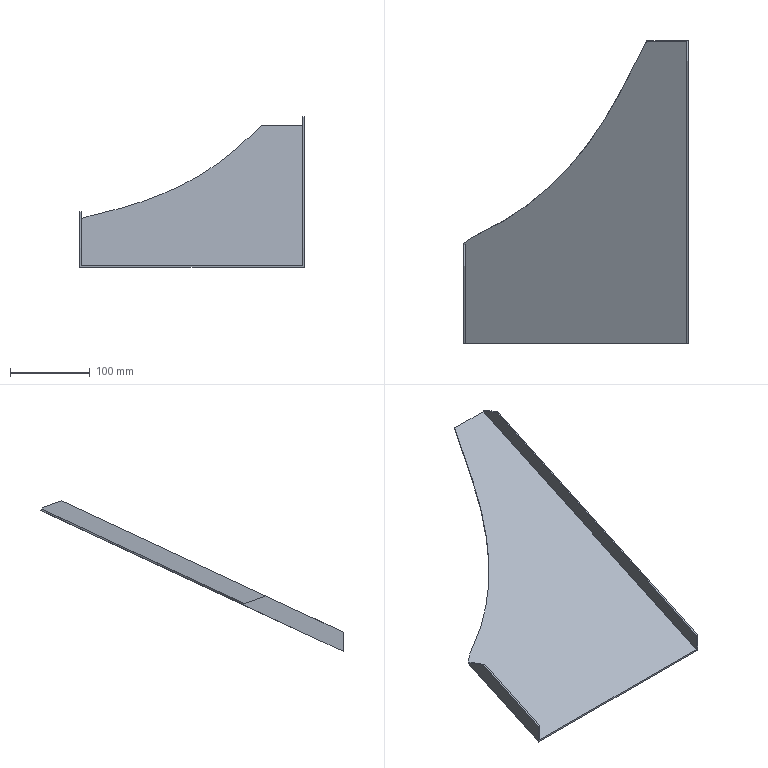Part | NX | features solid 2 | 1 solid | 13 faces | box 282.306 x 379.378 x 189.239 mm | volume 176482 mm3 | plane 12 | spline 1
STEP:
#1=CARTESIAN_POINT('',(299.694,-556.33,-245.421));
#2=VERTEX_POINT('',#1);
#3=CARTESIAN_POINT('',(297.694,-556.33,-245.421));
#4=VERTEX_POINT('',#3);
#5=CARTESIAN_POINT('',(337.694,-556.33,-245.421));
#6=DIRECTION('',(1.,0.,0.));
#7=VECTOR('',#6,1000.);
#8=LINE('',#5,#7);
#9=EDGE_CURVE('',#2,#4,#8,.F.);
#10=ORIENTED_EDGE('',*,*,#9,.F.);
#11=CARTESIAN_POINT('',(299.694,-680.,-303.09));
#12=VERTEX_POINT('',#11);
#13=CARTESIAN_POINT('',(299.694,-522.729,-229.753));
#14=DIRECTION('',(0.,-0.9063,-0.4226));
#15=VECTOR('',#14,1000.);
#16=LINE('',#13,#15);
#17=EDGE_CURVE('',#2,#12,#16,.T.);
#18=ORIENTED_EDGE('',*,*,#17,.T.);
#19=CARTESIAN_POINT('',(578.,-680.,-303.09));
#20=VERTEX_POINT('',#19);
#21=CARTESIAN_POINT('',(188.564,-680.,-303.09));
#22=DIRECTION('',(1.,0.,0.));
#23=VECTOR('',#22,1000.);
#24=LINE('',#21,#23);
#25=EDGE_CURVE('',#20,#12,#24,.F.);
#26=ORIENTED_EDGE('',*,*,#25,.F.);
#27=CARTESIAN_POINT('',(578.,-301.467,-126.577));
#28=VERTEX_POINT('',#27);
#29=CARTESIAN_POINT('',(578.,-522.729,-229.753));
#30=DIRECTION('',(0.,-0.9063,-0.4226));
#31=VECTOR('',#30,1000.);
#32=LINE('',#29,#31);
#33=EDGE_CURVE('',#28,#20,#32,.T.);
#34=ORIENTED_EDGE('',*,*,#33,.F.);
#35=CARTESIAN_POINT('',(527.431,-301.467,-126.577));
#36=VERTEX_POINT('',#35);
#37=CARTESIAN_POINT('',(570.,-301.467,-126.577));
#38=DIRECTION('',(-1.,0.,0.));
#39=VECTOR('',#38,1000.);
#40=LINE('',#37,#39);
#41=EDGE_CURVE('',#28,#36,#40,.T.);
#42=ORIENTED_EDGE('',*,*,#41,.T.);
#43=CARTESIAN_POINT('',(297.694,-555.03,-244.815));
#44=VERTEX_POINT('',#43);
#45=CARTESIAN_POINT('',(527.431,-301.467,-126.577));
#46=CARTESIAN_POINT('',(520.866,-314.161,-132.496));
#47=CARTESIAN_POINT('',(510.995,-333.189,-141.369));
#48=CARTESIAN_POINT('',(497.924,-358.611,-153.224));
#49=CARTESIAN_POINT('',(484.556,-383.863,-164.999));
#50=CARTESIAN_POINT('',(465.949,-414.249,-179.168));
#51=CARTESIAN_POINT('',(440.229,-448.639,-195.204));
#52=CARTESIAN_POINT('',(415.403,-475.145,-207.565));
#53=CARTESIAN_POINT('',(393.073,-494.953,-216.801));
#54=CARTESIAN_POINT('',(375.401,-508.723,-223.222));
#55=CARTESIAN_POINT('',(356.832,-521.362,-229.116));
#56=CARTESIAN_POINT('',(340.563,-530.912,-233.569));
#57=CARTESIAN_POINT('',(327.082,-537.971,-236.861));
#58=CARTESIAN_POINT('',(316.711,-542.944,-239.18));
#59=CARTESIAN_POINT('',(308.204,-547.256,-241.19));
#60=CARTESIAN_POINT('',(302.245,-551.756,-243.289));
#61=CARTESIAN_POINT('',(299.206,-553.933,-244.304));
#62=CARTESIAN_POINT('',(297.694,-555.03,-244.815));
#63=B_SPLINE_CURVE_WITH_KNOTS('',3,(#45,#46,#47,#48,#49,#50,#51,#52,#53,#54,#55,#56,#57,#58,#59,#60,#61,#62),.UNSPECIFIED.,.F.,.F.,(4,1,1,1,1,1,1,1,1,1,1,1,1,1,1,4),(0.9959,1.042,1.065,1.089,1.135,1.182,1.228,1.251,1.274,1.298,1.321,1.332,1.344,1.356,1.361,1.367),.UNSPECIFIED.);
#64=EDGE_CURVE('',#36,#44,#63,.T.);
#65=ORIENTED_EDGE('',*,*,#64,.T.);
#66=CARTESIAN_POINT('',(297.694,-522.729,-229.753));
#67=DIRECTION('',(0.,0.9063,0.4226));
#68=VECTOR('',#67,1000.);
#69=LINE('',#66,#68);
#70=EDGE_CURVE('',#4,#44,#69,.T.);
#71=ORIENTED_EDGE('',*,*,#70,.F.);
#72=EDGE_LOOP('',(#10,#18,#26,#34,#42,#65,#71));
#73=FACE_BOUND('',#72,.T.);
#74=CARTESIAN_POINT('',(337.694,-522.729,-229.753));
#75=DIRECTION('',(0.,-0.4226,0.9063));
#76=DIRECTION('',(1.,0.,0.));
#77=AXIS2_PLACEMENT_3D('',#74,#75,#76);
#78=PLANE('',#77);
#79=ADVANCED_FACE('',(#73),#78,.T.);
#80=CARTESIAN_POINT('',(578.,-302.312,-124.764));
#81=VERTEX_POINT('',#80);
#82=CARTESIAN_POINT('',(578.,-301.467,-126.577));
#83=DIRECTION('',(0.,-0.4226,0.9063));
#84=VECTOR('',#83,1000.);
#85=LINE('',#82,#84);
#86=EDGE_CURVE('',#28,#81,#85,.T.);
#87=ORIENTED_EDGE('',*,*,#86,.T.);
#88=CARTESIAN_POINT('',(580.,-302.312,-124.764));
#89=VERTEX_POINT('',#88);
#90=CARTESIAN_POINT('',(570.,-302.312,-124.764));
#91=DIRECTION('',(1.,0.,0.));
#92=VECTOR('',#91,1000.);
#93=LINE('',#90,#92);
#94=EDGE_CURVE('',#81,#89,#93,.T.);
#95=ORIENTED_EDGE('',*,*,#94,.T.);
#96=CARTESIAN_POINT('',(580.,-300.622,-128.389));
#97=VERTEX_POINT('',#96);
#98=CARTESIAN_POINT('',(580.,-301.467,-126.577));
#99=DIRECTION('',(0.,0.4226,-0.9063));
#100=VECTOR('',#99,1000.);
#101=LINE('',#98,#100);
#102=EDGE_CURVE('',#89,#97,#101,.T.);
#103=ORIENTED_EDGE('',*,*,#102,.T.);
#104=CARTESIAN_POINT('',(527.869,-300.622,-128.389));
#105=VERTEX_POINT('',#104);
#106=CARTESIAN_POINT('',(570.,-300.622,-128.389));
#107=DIRECTION('',(-1.,0.,0.));
#108=VECTOR('',#107,1000.);
#109=LINE('',#106,#108);
#110=EDGE_CURVE('',#97,#105,#109,.T.);
#111=ORIENTED_EDGE('',*,*,#110,.T.);
#112=CARTESIAN_POINT('',(527.431,-301.467,-126.577));
#113=CARTESIAN_POINT('',(527.577,-301.185,-127.181));
#114=CARTESIAN_POINT('',(527.723,-300.903,-127.785));
#115=CARTESIAN_POINT('',(527.869,-300.622,-128.389));
#116=B_SPLINE_CURVE_WITH_KNOTS('',3,(#112,#113,#114,#115),.UNSPECIFIED.,.F.,.F.,(4,4),(0.07876,0.08081),.UNSPECIFIED.);
#117=EDGE_CURVE('',#36,#105,#116,.T.);
#118=ORIENTED_EDGE('',*,*,#117,.F.);
#119=ORIENTED_EDGE('',*,*,#41,.F.);
#120=EDGE_LOOP('',(#87,#95,#103,#111,#118,#119));
#121=FACE_BOUND('',#120,.T.);
#122=CARTESIAN_POINT('',(570.,-301.467,-126.577));
#123=DIRECTION('',(0.,-0.9063,-0.4226));
#124=DIRECTION('',(0.,0.4226,-0.9063));
#125=AXIS2_PLACEMENT_3D('',#122,#123,#124);
#126=PLANE('',#125);
#127=ADVANCED_FACE('',(#121),#126,.F.);
#128=CARTESIAN_POINT('',(297.694,-555.03,-247.022));
#129=VERTEX_POINT('',#128);
#130=CARTESIAN_POINT('',(527.869,-300.622,-128.389));
#131=CARTESIAN_POINT('',(521.294,-313.334,-134.317));
#132=CARTESIAN_POINT('',(511.409,-332.39,-143.203));
#133=CARTESIAN_POINT('',(498.317,-357.846,-155.074));
#134=CARTESIAN_POINT('',(484.961,-383.152,-166.874));
#135=CARTESIAN_POINT('',(466.378,-413.617,-181.08));
#136=CARTESIAN_POINT('',(440.678,-448.104,-197.161));
#137=CARTESIAN_POINT('',(415.858,-474.699,-209.563));
#138=CARTESIAN_POINT('',(393.532,-494.571,-218.83));
#139=CARTESIAN_POINT('',(375.839,-508.405,-225.281));
#140=CARTESIAN_POINT('',(357.211,-521.124,-231.212));
#141=CARTESIAN_POINT('',(340.857,-530.75,-235.7));
#142=CARTESIAN_POINT('',(327.286,-537.87,-239.02));
#143=CARTESIAN_POINT('',(316.84,-542.884,-241.358));
#144=CARTESIAN_POINT('',(308.261,-547.216,-243.378));
#145=CARTESIAN_POINT('',(302.27,-551.738,-245.487));
#146=CARTESIAN_POINT('',(299.214,-553.927,-246.508));
#147=CARTESIAN_POINT('',(297.694,-555.03,-247.022));
#148=B_SPLINE_CURVE_WITH_KNOTS('',3,(#130,#131,#132,#133,#134,#135,#136,#137,#138,#139,#140,#141,#142,#143,#144,#145,#146,#147),.UNSPECIFIED.,.F.,.F.,(4,1,1,1,1,1,1,1,1,1,1,1,1,1,1,4),(-0.06545,-0.01955,0.003406,0.02636,0.07226,0.1182,0.1641,0.187,0.21,0.2329,0.2559,0.2674,0.2788,0.2903,0.2961,0.3018),.UNSPECIFIED.);
#149=EDGE_CURVE('',#105,#129,#148,.T.);
#150=ORIENTED_EDGE('',*,*,#149,.T.);
#151=CARTESIAN_POINT('',(297.694,-555.03,-235.335));
#152=DIRECTION('',(0.,0.,1.));
#153=VECTOR('',#152,1000.);
#154=LINE('',#151,#153);
#155=EDGE_CURVE('',#44,#129,#154,.F.);
#156=ORIENTED_EDGE('',*,*,#155,.F.);
#157=ORIENTED_EDGE('',*,*,#64,.F.);
#158=ORIENTED_EDGE('',*,*,#117,.T.);
#159=EDGE_LOOP('',(#150,#156,#157,#158));
#160=FACE_BOUND('',#159,.T.);
#161=CARTESIAN_POINT('',(528.87,-298.685,-247.745));
#162=CARTESIAN_POINT('',(528.87,-298.685,-125.854));
#163=CARTESIAN_POINT('',(521.874,-312.214,-247.745));
#164=CARTESIAN_POINT('',(521.874,-312.214,-125.854));
#165=CARTESIAN_POINT('',(511.363,-332.465,-247.745));
#166=CARTESIAN_POINT('',(511.363,-332.465,-125.854));
#167=CARTESIAN_POINT('',(497.414,-359.617,-247.745));
#168=CARTESIAN_POINT('',(497.414,-359.617,-125.854));
#169=CARTESIAN_POINT('',(483.345,-386.039,-247.745));
#170=CARTESIAN_POINT('',(483.345,-386.039,-125.854));
#171=CARTESIAN_POINT('',(463.62,-417.783,-247.745));
#172=CARTESIAN_POINT('',(463.62,-417.783,-125.854));
#173=CARTESIAN_POINT('',(436.439,-453.196,-247.745));
#174=CARTESIAN_POINT('',(436.439,-453.196,-125.854));
#175=CARTESIAN_POINT('',(410.556,-479.827,-247.745));
#176=CARTESIAN_POINT('',(410.556,-479.827,-125.854));
#177=CARTESIAN_POINT('',(388.011,-499.079,-247.745));
#178=CARTESIAN_POINT('',(388.011,-499.079,-125.854));
#179=CARTESIAN_POINT('',(373.197,-510.191,-247.745));
#180=CARTESIAN_POINT('',(373.197,-510.191,-125.854));
#181=CARTESIAN_POINT('',(360.944,-518.489,-247.745));
#182=CARTESIAN_POINT('',(360.944,-518.489,-125.854));
#183=CARTESIAN_POINT('',(351.559,-524.409,-247.745));
#184=CARTESIAN_POINT('',(351.559,-524.409,-125.854));
#185=CARTESIAN_POINT('',(341.997,-530.012,-247.745));
#186=CARTESIAN_POINT('',(341.997,-530.012,-125.854));
#187=CARTESIAN_POINT('',(332.196,-535.345,-247.745));
#188=CARTESIAN_POINT('',(332.196,-535.345,-125.854));
#189=CARTESIAN_POINT('',(324.009,-539.443,-247.745));
#190=CARTESIAN_POINT('',(324.009,-539.443,-125.854));
#191=CARTESIAN_POINT('',(317.085,-542.786,-247.745));
#192=CARTESIAN_POINT('',(317.085,-542.786,-125.854));
#193=CARTESIAN_POINT('',(312.134,-545.294,-247.745));
#194=CARTESIAN_POINT('',(312.134,-545.294,-125.854));
#195=CARTESIAN_POINT('',(307.693,-547.779,-247.745));
#196=CARTESIAN_POINT('',(307.693,-547.779,-125.854));
#197=CARTESIAN_POINT('',(304.351,-550.197,-247.745));
#198=CARTESIAN_POINT('',(304.351,-550.197,-125.854));
#199=CARTESIAN_POINT('',(301.025,-552.614,-247.745));
#200=CARTESIAN_POINT('',(301.025,-552.614,-125.854));
#201=CARTESIAN_POINT('',(298.804,-554.225,-247.745));
#202=CARTESIAN_POINT('',(298.804,-554.225,-125.854));
#203=CARTESIAN_POINT('',(297.694,-555.03,-247.745));
#204=CARTESIAN_POINT('',(297.694,-555.03,-125.854));
#205=B_SPLINE_SURFACE_WITH_KNOTS('',3,1,((#161,#162),(#163,#164),(#165,#166),(#167,#168),(#169,#170),(#171,#172),(#173,#174),(#175,#176),(#177,#178),(#179,#180),(#181,#182),(#183,#184),(#185,#186),(#187,#188),(#189,#190),(#191,#192),(#193,#194),(#195,#196),(#197,#198),(#199,#200),(#201,#202),(#203,#204)),.SURF_OF_LINEAR_EXTRUSION.,.F.,.F.,.F.,(4,1,1,1,1,1,1,1,1,1,1,1,1,1,1,1,1,1,1,4),(2,2),(-0.004215,0.1262,0.1914,0.2566,0.387,0.5174,0.6478,0.713,0.7782,0.8108,0.8434,0.876,0.9086,0.9412,0.9575,0.9738,0.9901,1.006,1.023,1.039),(0.,1.),.UNSPECIFIED.);
#206=ADVANCED_FACE('',(#160),#205,.T.);
#207=CARTESIAN_POINT('',(297.694,-680.,-305.297));
#208=VERTEX_POINT('',#207);
#209=CARTESIAN_POINT('',(297.694,-479.94,-212.007));
#210=DIRECTION('',(0.,-0.9063,-0.4226));
#211=VECTOR('',#210,1000.);
#212=LINE('',#209,#211);
#213=EDGE_CURVE('',#129,#208,#212,.T.);
#214=ORIENTED_EDGE('',*,*,#213,.T.);
#215=CARTESIAN_POINT('',(297.694,-680.,-281.022));
#216=VERTEX_POINT('',#215);
#217=CARTESIAN_POINT('',(297.694,-680.,-210.194));
#218=DIRECTION('',(0.,0.,1.));
#219=VECTOR('',#218,1000.);
#220=LINE('',#217,#219);
#221=EDGE_CURVE('',#216,#208,#220,.F.);
#222=ORIENTED_EDGE('',*,*,#221,.F.);
#223=CARTESIAN_POINT('',(297.694,-582.908,-235.748));
#224=VERTEX_POINT('',#223);
#225=CARTESIAN_POINT('',(297.694,-564.782,-227.295));
#226=DIRECTION('',(0.,-0.9063,-0.4226));
#227=VECTOR('',#226,1000.);
#228=LINE('',#225,#227);
#229=EDGE_CURVE('',#224,#216,#228,.T.);
#230=ORIENTED_EDGE('',*,*,#229,.F.);
#231=CARTESIAN_POINT('',(297.694,-582.908,-235.748));
#232=DIRECTION('',(0.,-0.9397,0.342));
#233=VECTOR('',#232,1000.);
#234=LINE('',#231,#233);
#235=EDGE_CURVE('',#224,#4,#234,.F.);
#236=ORIENTED_EDGE('',*,*,#235,.T.);
#237=ORIENTED_EDGE('',*,*,#70,.T.);
#238=ORIENTED_EDGE('',*,*,#155,.T.);
#239=EDGE_LOOP('',(#214,#222,#230,#236,#237,#238));
#240=FACE_BOUND('',#239,.T.);
#241=CARTESIAN_POINT('',(297.694,-480.785,-210.194));
#242=DIRECTION('',(1.,0.,0.));
#243=DIRECTION('',(0.,1.,0.));
#244=AXIS2_PLACEMENT_3D('',#241,#242,#243);
#245=PLANE('',#244);
#246=ADVANCED_FACE('',(#240),#245,.F.);
#247=CARTESIAN_POINT('',(580.,-680.,-305.297));
#248=VERTEX_POINT('',#247);
#249=CARTESIAN_POINT('',(188.564,-680.,-305.297));
#250=DIRECTION('',(1.,0.,0.));
#251=VECTOR('',#250,1000.);
#252=LINE('',#249,#251);
#253=EDGE_CURVE('',#248,#208,#252,.F.);
#254=ORIENTED_EDGE('',*,*,#253,.F.);
#255=CARTESIAN_POINT('',(580.,-680.,-281.022));
#256=VERTEX_POINT('',#255);
#257=CARTESIAN_POINT('',(580.,-680.,234.426));
#258=DIRECTION('',(0.,0.,1.));
#259=VECTOR('',#258,1000.);
#260=LINE('',#257,#259);
#261=EDGE_CURVE('',#256,#248,#260,.F.);
#262=ORIENTED_EDGE('',*,*,#261,.F.);
#263=CARTESIAN_POINT('',(578.,-680.,-281.022));
#264=VERTEX_POINT('',#263);
#265=CARTESIAN_POINT('',(570.,-680.,-281.022));
#266=DIRECTION('',(1.,0.,0.));
#267=VECTOR('',#266,1000.);
#268=LINE('',#265,#267);
#269=EDGE_CURVE('',#264,#256,#268,.T.);
#270=ORIENTED_EDGE('',*,*,#269,.F.);
#271=CARTESIAN_POINT('',(578.,-680.,-151.934));
#272=DIRECTION('',(0.,0.,-1.));
#273=VECTOR('',#272,1000.);
#274=LINE('',#271,#273);
#275=EDGE_CURVE('',#20,#264,#274,.F.);
#276=ORIENTED_EDGE('',*,*,#275,.F.);
#277=ORIENTED_EDGE('',*,*,#25,.T.);
#278=CARTESIAN_POINT('',(299.694,-680.,-281.022));
#279=VERTEX_POINT('',#278);
#280=CARTESIAN_POINT('',(299.694,-680.,-245.421));
#281=DIRECTION('',(0.,0.,-1.));
#282=VECTOR('',#281,1000.);
#283=LINE('',#280,#282);
#284=EDGE_CURVE('',#12,#279,#283,.F.);
#285=ORIENTED_EDGE('',*,*,#284,.T.);
#286=CARTESIAN_POINT('',(188.564,-680.,-281.022));
#287=DIRECTION('',(-1.,0.,0.));
#288=VECTOR('',#287,1000.);
#289=LINE('',#286,#288);
#290=EDGE_CURVE('',#279,#216,#289,.T.);
#291=ORIENTED_EDGE('',*,*,#290,.T.);
#292=ORIENTED_EDGE('',*,*,#221,.T.);
#293=EDGE_LOOP('',(#254,#262,#270,#276,#277,#285,#291,#292));
#294=FACE_BOUND('',#293,.T.);
#295=CARTESIAN_POINT('',(188.564,-680.,-430.));
#296=DIRECTION('',(0.,1.,0.));
#297=DIRECTION('',(-1.,0.,0.));
#298=AXIS2_PLACEMENT_3D('',#295,#296,#297);
#299=PLANE('',#298);
#300=ADVANCED_FACE('',(#294),#299,.F.);
#301=ORIENTED_EDGE('',*,*,#102,.F.);
#302=CARTESIAN_POINT('',(580.,-326.233,-116.058));
#303=VERTEX_POINT('',#302);
#304=CARTESIAN_POINT('',(580.,266.605,-331.833));
#305=DIRECTION('',(0.,0.9397,-0.342));
#306=VECTOR('',#305,1000.);
#307=LINE('',#304,#306);
#308=EDGE_CURVE('',#89,#303,#307,.F.);
#309=ORIENTED_EDGE('',*,*,#308,.T.);
#310=CARTESIAN_POINT('',(580.,464.254,252.552));
#311=DIRECTION('',(0.,0.9063,0.4226));
#312=VECTOR('',#311,1000.);
#313=LINE('',#310,#312);
#314=EDGE_CURVE('',#303,#256,#313,.F.);
#315=ORIENTED_EDGE('',*,*,#314,.T.);
#316=ORIENTED_EDGE('',*,*,#261,.T.);
#317=CARTESIAN_POINT('',(580.,473.552,232.614));
#318=DIRECTION('',(0.,-0.9063,-0.4226));
#319=VECTOR('',#318,1000.);
#320=LINE('',#317,#319);
#321=EDGE_CURVE('',#97,#248,#320,.T.);
#322=ORIENTED_EDGE('',*,*,#321,.F.);
#323=EDGE_LOOP('',(#301,#309,#315,#316,#322));
#324=FACE_BOUND('',#323,.T.);
#325=CARTESIAN_POINT('',(580.,472.707,234.426));
#326=DIRECTION('',(1.,0.,0.));
#327=DIRECTION('',(0.,0.,-1.));
#328=AXIS2_PLACEMENT_3D('',#325,#326,#327);
#329=PLANE('',#328);
#330=ADVANCED_FACE('',(#324),#329,.T.);
#331=ORIENTED_EDGE('',*,*,#110,.F.);
#332=ORIENTED_EDGE('',*,*,#321,.T.);
#333=ORIENTED_EDGE('',*,*,#253,.T.);
#334=ORIENTED_EDGE('',*,*,#213,.F.);
#335=ORIENTED_EDGE('',*,*,#149,.F.);
#336=EDGE_LOOP('',(#331,#332,#333,#334,#335));
#337=FACE_BOUND('',#336,.T.);
#338=CARTESIAN_POINT('',(337.694,-521.883,-231.565));
#339=DIRECTION('',(0.,-0.4226,0.9063));
#340=DIRECTION('',(1.,0.,0.));
#341=AXIS2_PLACEMENT_3D('',#338,#339,#340);
#342=PLANE('',#341);
#343=ADVANCED_FACE('',(#337),#342,.F.);
#344=ORIENTED_EDGE('',*,*,#314,.F.);
#345=CARTESIAN_POINT('',(578.,-326.233,-116.058));
#346=VERTEX_POINT('',#345);
#347=CARTESIAN_POINT('',(568.,-326.233,-116.058));
#348=DIRECTION('',(1.,0.,0.));
#349=VECTOR('',#348,1000.);
#350=LINE('',#347,#349);
#351=EDGE_CURVE('',#303,#346,#350,.F.);
#352=ORIENTED_EDGE('',*,*,#351,.T.);
#353=CARTESIAN_POINT('',(578.,-364.298,-133.808));
#354=DIRECTION('',(0.,0.9063,0.4226));
#355=VECTOR('',#354,1000.);
#356=LINE('',#353,#355);
#357=EDGE_CURVE('',#346,#264,#356,.F.);
#358=ORIENTED_EDGE('',*,*,#357,.T.);
#359=ORIENTED_EDGE('',*,*,#269,.T.);
#360=EDGE_LOOP('',(#344,#352,#358,#359));
#361=FACE_BOUND('',#360,.T.);
#362=CARTESIAN_POINT('',(570.,-364.298,-133.808));
#363=DIRECTION('',(0.,0.4226,-0.9063));
#364=DIRECTION('',(0.,-0.9063,-0.4226));
#365=AXIS2_PLACEMENT_3D('',#362,#363,#364);
#366=PLANE('',#365);
#367=ADVANCED_FACE('',(#361),#366,.F.);
#368=ORIENTED_EDGE('',*,*,#357,.F.);
#369=CARTESIAN_POINT('',(578.,-340.851,-110.737));
#370=DIRECTION('',(0.,-0.9397,0.342));
#371=VECTOR('',#370,1000.);
#372=LINE('',#369,#371);
#373=EDGE_CURVE('',#346,#81,#372,.F.);
#374=ORIENTED_EDGE('',*,*,#373,.T.);
#375=ORIENTED_EDGE('',*,*,#86,.F.);
#376=ORIENTED_EDGE('',*,*,#33,.T.);
#377=ORIENTED_EDGE('',*,*,#275,.T.);
#378=EDGE_LOOP('',(#368,#374,#375,#376,#377));
#379=FACE_BOUND('',#378,.T.);
#380=CARTESIAN_POINT('',(578.,-355.845,-151.934));
#381=DIRECTION('',(-1.,0.,0.));
#382=DIRECTION('',(0.,0.,1.));
#383=AXIS2_PLACEMENT_3D('',#380,#381,#382);
#384=PLANE('',#383);
#385=ADVANCED_FACE('',(#379),#384,.T.);
#386=CARTESIAN_POINT('',(299.694,-582.908,-235.748));
#387=VERTEX_POINT('',#386);
#388=CARTESIAN_POINT('',(299.694,-564.782,-227.295));
#389=DIRECTION('',(0.,-0.9063,-0.4226));
#390=VECTOR('',#389,1000.);
#391=LINE('',#388,#390);
#392=EDGE_CURVE('',#387,#279,#391,.T.);
#393=ORIENTED_EDGE('',*,*,#392,.F.);
#394=CARTESIAN_POINT('',(337.694,-582.908,-235.748));
#395=DIRECTION('',(-1.,0.,0.));
#396=VECTOR('',#395,1000.);
#397=LINE('',#394,#396);
#398=EDGE_CURVE('',#387,#224,#397,.T.);
#399=ORIENTED_EDGE('',*,*,#398,.T.);
#400=ORIENTED_EDGE('',*,*,#229,.T.);
#401=ORIENTED_EDGE('',*,*,#290,.F.);
#402=EDGE_LOOP('',(#393,#399,#400,#401));
#403=FACE_BOUND('',#402,.T.);
#404=CARTESIAN_POINT('',(337.694,-564.782,-227.295));
#405=DIRECTION('',(0.,0.4226,-0.9063));
#406=DIRECTION('',(0.,-0.9063,-0.4226));
#407=AXIS2_PLACEMENT_3D('',#404,#405,#406);
#408=PLANE('',#407);
#409=ADVANCED_FACE('',(#403),#408,.F.);
#410=ORIENTED_EDGE('',*,*,#17,.F.);
#411=CARTESIAN_POINT('',(299.694,-582.908,-235.748));
#412=DIRECTION('',(0.,0.9397,-0.342));
#413=VECTOR('',#412,1000.);
#414=LINE('',#411,#413);
#415=EDGE_CURVE('',#2,#387,#414,.F.);
#416=ORIENTED_EDGE('',*,*,#415,.T.);
#417=ORIENTED_EDGE('',*,*,#392,.T.);
#418=ORIENTED_EDGE('',*,*,#284,.F.);
#419=EDGE_LOOP('',(#410,#416,#417,#418));
#420=FACE_BOUND('',#419,.T.);
#421=CARTESIAN_POINT('',(299.694,-556.33,-245.421));
#422=DIRECTION('',(-1.,0.,0.));
#423=DIRECTION('',(0.,-1.,0.));
#424=AXIS2_PLACEMENT_3D('',#421,#422,#423);
#425=PLANE('',#424);
#426=ADVANCED_FACE('',(#420),#425,.F.);
#427=ORIENTED_EDGE('',*,*,#415,.F.);
#428=ORIENTED_EDGE('',*,*,#9,.T.);
#429=ORIENTED_EDGE('',*,*,#235,.F.);
#430=ORIENTED_EDGE('',*,*,#398,.F.);
#431=EDGE_LOOP('',(#427,#428,#429,#430));
#432=FACE_BOUND('',#431,.T.);
#433=CARTESIAN_POINT('',(337.694,-582.908,-235.748));
#434=DIRECTION('',(0.,-0.342,-0.9397));
#435=DIRECTION('',(0.,0.9397,-0.342));
#436=AXIS2_PLACEMENT_3D('',#433,#434,#435);
#437=PLANE('',#436);
#438=ADVANCED_FACE('',(#432),#437,.F.);
#439=ORIENTED_EDGE('',*,*,#308,.F.);
#440=ORIENTED_EDGE('',*,*,#94,.F.);
#441=ORIENTED_EDGE('',*,*,#373,.F.);
#442=ORIENTED_EDGE('',*,*,#351,.F.);
#443=EDGE_LOOP('',(#439,#440,#441,#442));
#444=FACE_BOUND('',#443,.T.);
#445=CARTESIAN_POINT('',(570.,-326.233,-116.058));
#446=DIRECTION('',(0.,-0.342,-0.9397));
#447=DIRECTION('',(0.,0.9397,-0.342));
#448=AXIS2_PLACEMENT_3D('',#445,#446,#447);
#449=PLANE('',#448);
#450=ADVANCED_FACE('',(#444),#449,.F.);
#451=CLOSED_SHELL('',(#79,#127,#206,#246,#300,#330,#343,#367,#385,#409,#426,#438,#450));
#452=MANIFOLD_SOLID_BREP('',#451);
#453=(LENGTH_UNIT()NAMED_UNIT(*)SI_UNIT(.MILLI.,.METRE.));
#454=UNCERTAINTY_MEASURE_WITH_UNIT(LENGTH_MEASURE(0.0508),#453,'','');
#455=(NAMED_UNIT(*)PLANE_ANGLE_UNIT()SI_UNIT($,.RADIAN.));
#456=(NAMED_UNIT(*)SI_UNIT($,.STERADIAN.)SOLID_ANGLE_UNIT());
#457=(GEOMETRIC_REPRESENTATION_CONTEXT(3)GLOBAL_UNCERTAINTY_ASSIGNED_CONTEXT((#454))GLOBAL_UNIT_ASSIGNED_CONTEXT((#453,#455,#456))REPRESENTATION_CONTEXT('',''));
#458=ADVANCED_BREP_SHAPE_REPRESENTATION('',(#452),#457);